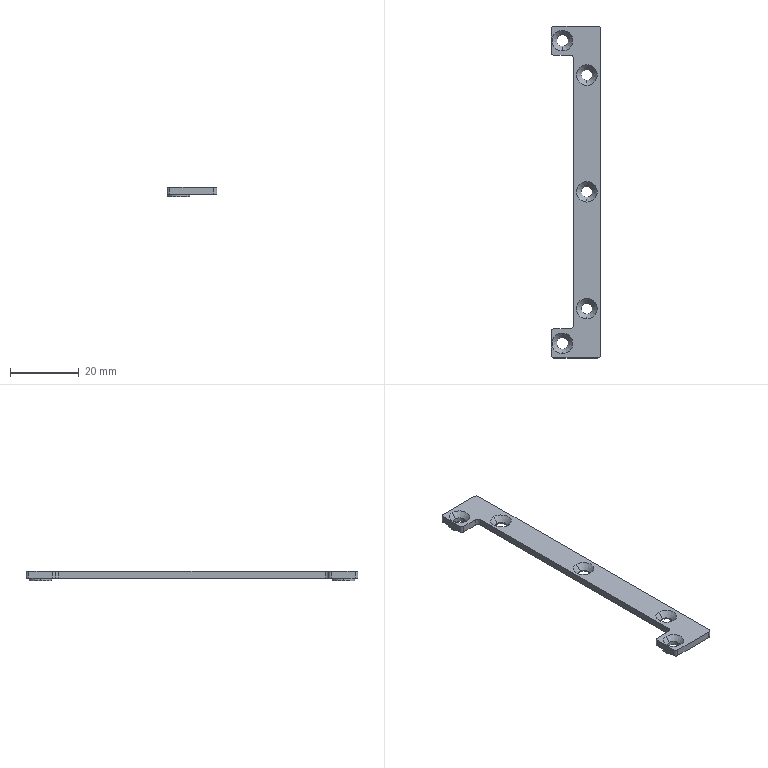Part | 1 solid | 44 faces | box 14.52 x 96.5 x 2.7 mm | volume 1629 mm3 | cylinder 22 | plane 12 | cone 10 | commonest cylinder face diameters 3.2 x6 1.6 x4 2 x4 3.4 x4 6.6 x4
STEP:
#1=CARTESIAN_POINT('',(-7.26,47.45,-2.));
#2=VERTEX_POINT('',#1);
#3=CARTESIAN_POINT('',(-7.26,44.,-2.));
#4=VERTEX_POINT('',#3);
#5=CARTESIAN_POINT('',(-7.26,47.45,-2.));
#6=DIRECTION('',(0.,-1.,0.));
#7=VECTOR('',#6,1000.);
#8=LINE('',#5,#7);
#9=EDGE_CURVE('',#2,#4,#8,.T.);
#10=ORIENTED_EDGE('',*,*,#9,.F.);
#11=CARTESIAN_POINT('',(-6.46,48.25,-2.));
#12=VERTEX_POINT('',#11);
#13=CARTESIAN_POINT('',(-6.46,47.45,-2.));
#14=DIRECTION('',(0.,0.,1.));
#15=DIRECTION('',(0.,1.,0.));
#16=AXIS2_PLACEMENT_3D('',#13,#14,#15);
#17=CIRCLE('',#16,0.8);
#18=EDGE_CURVE('',#12,#2,#17,.T.);
#19=ORIENTED_EDGE('',*,*,#18,.F.);
#20=CARTESIAN_POINT('',(6.26,48.25,-2.));
#21=VERTEX_POINT('',#20);
#22=CARTESIAN_POINT('',(6.26,48.25,-2.));
#23=DIRECTION('',(-1.,0.,0.));
#24=VECTOR('',#23,1000.);
#25=LINE('',#22,#24);
#26=EDGE_CURVE('',#21,#12,#25,.T.);
#27=ORIENTED_EDGE('',*,*,#26,.F.);
#28=CARTESIAN_POINT('',(7.26,47.25,-2.));
#29=VERTEX_POINT('',#28);
#30=CARTESIAN_POINT('',(6.26,47.25,-2.));
#31=DIRECTION('',(0.,0.,-1.));
#32=DIRECTION('',(0.,1.,0.));
#33=AXIS2_PLACEMENT_3D('',#30,#31,#32);
#34=CIRCLE('',#33,1.);
#35=EDGE_CURVE('',#21,#29,#34,.T.);
#36=ORIENTED_EDGE('',*,*,#35,.T.);
#37=CARTESIAN_POINT('',(7.26,-47.25,-2.));
#38=VERTEX_POINT('',#37);
#39=CARTESIAN_POINT('',(7.26,-47.25,-2.));
#40=DIRECTION('',(0.,1.,0.));
#41=VECTOR('',#40,1000.);
#42=LINE('',#39,#41);
#43=EDGE_CURVE('',#38,#29,#42,.T.);
#44=ORIENTED_EDGE('',*,*,#43,.F.);
#45=CARTESIAN_POINT('',(6.26,-48.25,-2.));
#46=VERTEX_POINT('',#45);
#47=CARTESIAN_POINT('',(6.26,-47.25,-2.));
#48=DIRECTION('',(0.,0.,-1.));
#49=DIRECTION('',(1.,0.,0.));
#50=AXIS2_PLACEMENT_3D('',#47,#48,#49);
#51=CIRCLE('',#50,1.);
#52=EDGE_CURVE('',#38,#46,#51,.T.);
#53=ORIENTED_EDGE('',*,*,#52,.T.);
#54=CARTESIAN_POINT('',(-6.46,-48.25,-2.));
#55=VERTEX_POINT('',#54);
#56=CARTESIAN_POINT('',(-6.46,-48.25,-2.));
#57=DIRECTION('',(1.,0.,0.));
#58=VECTOR('',#57,1000.);
#59=LINE('',#56,#58);
#60=EDGE_CURVE('',#55,#46,#59,.T.);
#61=ORIENTED_EDGE('',*,*,#60,.F.);
#62=CARTESIAN_POINT('',(-7.26,-47.45,-2.));
#63=VERTEX_POINT('',#62);
#64=CARTESIAN_POINT('',(-6.46,-47.45,-2.));
#65=DIRECTION('',(0.,0.,1.));
#66=DIRECTION('',(-1.,0.,0.));
#67=AXIS2_PLACEMENT_3D('',#64,#65,#66);
#68=CIRCLE('',#67,0.8);
#69=EDGE_CURVE('',#63,#55,#68,.T.);
#70=ORIENTED_EDGE('',*,*,#69,.F.);
#71=CARTESIAN_POINT('',(-7.26,-44.,-2.));
#72=VERTEX_POINT('',#71);
#73=CARTESIAN_POINT('',(-7.26,-44.,-2.));
#74=DIRECTION('',(0.,-1.,0.));
#75=VECTOR('',#74,1000.);
#76=LINE('',#73,#75);
#77=EDGE_CURVE('',#72,#63,#76,.T.);
#78=ORIENTED_EDGE('',*,*,#77,.F.);
#79=CARTESIAN_POINT('',(-0.66,-44.,-2.));
#80=VERTEX_POINT('',#79);
#81=CARTESIAN_POINT('',(-3.96,-44.,-2.));
#82=DIRECTION('',(0.,0.,-1.));
#83=DIRECTION('',(1.,0.,0.));
#84=AXIS2_PLACEMENT_3D('',#81,#82,#83);
#85=CIRCLE('',#84,3.3);
#86=EDGE_CURVE('',#80,#72,#85,.T.);
#87=ORIENTED_EDGE('',*,*,#86,.F.);
#88=CARTESIAN_POINT('',(-3.96,-44.,-2.));
#89=DIRECTION('',(0.,0.,-1.));
#90=DIRECTION('',(-1.,0.,0.));
#91=AXIS2_PLACEMENT_3D('',#88,#89,#90);
#92=CIRCLE('',#91,3.3);
#93=EDGE_CURVE('',#72,#80,#92,.T.);
#94=ORIENTED_EDGE('',*,*,#93,.F.);
#95=CARTESIAN_POINT('',(-7.26,-40.55,-2.));
#96=VERTEX_POINT('',#95);
#97=CARTESIAN_POINT('',(-7.26,-40.55,-2.));
#98=DIRECTION('',(0.,-1.,0.));
#99=VECTOR('',#98,1000.);
#100=LINE('',#97,#99);
#101=EDGE_CURVE('',#96,#72,#100,.T.);
#102=ORIENTED_EDGE('',*,*,#101,.F.);
#103=CARTESIAN_POINT('',(-6.46,-39.75,-2.));
#104=VERTEX_POINT('',#103);
#105=CARTESIAN_POINT('',(-6.46,-40.55,-2.));
#106=DIRECTION('',(0.,0.,1.));
#107=DIRECTION('',(0.,1.,0.));
#108=AXIS2_PLACEMENT_3D('',#105,#106,#107);
#109=CIRCLE('',#108,0.8);
#110=EDGE_CURVE('',#104,#96,#109,.T.);
#111=ORIENTED_EDGE('',*,*,#110,.F.);
#112=CARTESIAN_POINT('',(-1.66,-39.75,-2.));
#113=VERTEX_POINT('',#112);
#114=CARTESIAN_POINT('',(-1.66,-39.75,-2.));
#115=DIRECTION('',(-1.,0.,0.));
#116=VECTOR('',#115,1000.);
#117=LINE('',#114,#116);
#118=EDGE_CURVE('',#113,#104,#117,.T.);
#119=ORIENTED_EDGE('',*,*,#118,.F.);
#120=CARTESIAN_POINT('',(-0.66,-38.75,-2.));
#121=VERTEX_POINT('',#120);
#122=CARTESIAN_POINT('',(-1.66,-38.75,-2.));
#123=DIRECTION('',(0.,0.,1.));
#124=DIRECTION('',(0.,-1.,0.));
#125=AXIS2_PLACEMENT_3D('',#122,#123,#124);
#126=CIRCLE('',#125,1.);
#127=EDGE_CURVE('',#113,#121,#126,.T.);
#128=ORIENTED_EDGE('',*,*,#127,.T.);
#129=CARTESIAN_POINT('',(-0.66,38.75,-2.));
#130=VERTEX_POINT('',#129);
#131=CARTESIAN_POINT('',(-0.66,38.75,-2.));
#132=DIRECTION('',(0.,-1.,0.));
#133=VECTOR('',#132,1000.);
#134=LINE('',#131,#133);
#135=EDGE_CURVE('',#130,#121,#134,.T.);
#136=ORIENTED_EDGE('',*,*,#135,.F.);
#137=CARTESIAN_POINT('',(-1.66,39.75,-2.));
#138=VERTEX_POINT('',#137);
#139=CARTESIAN_POINT('',(-1.66,38.75,-2.));
#140=DIRECTION('',(0.,0.,1.));
#141=DIRECTION('',(1.,0.,0.));
#142=AXIS2_PLACEMENT_3D('',#139,#140,#141);
#143=CIRCLE('',#142,1.);
#144=EDGE_CURVE('',#130,#138,#143,.T.);
#145=ORIENTED_EDGE('',*,*,#144,.T.);
#146=CARTESIAN_POINT('',(-6.46,39.75,-2.));
#147=VERTEX_POINT('',#146);
#148=CARTESIAN_POINT('',(-6.46,39.75,-2.));
#149=DIRECTION('',(1.,0.,0.));
#150=VECTOR('',#149,1000.);
#151=LINE('',#148,#150);
#152=EDGE_CURVE('',#147,#138,#151,.T.);
#153=ORIENTED_EDGE('',*,*,#152,.F.);
#154=CARTESIAN_POINT('',(-7.26,40.55,-2.));
#155=VERTEX_POINT('',#154);
#156=CARTESIAN_POINT('',(-6.46,40.55,-2.));
#157=DIRECTION('',(0.,0.,1.));
#158=DIRECTION('',(-1.,0.,0.));
#159=AXIS2_PLACEMENT_3D('',#156,#157,#158);
#160=CIRCLE('',#159,0.8);
#161=EDGE_CURVE('',#155,#147,#160,.T.);
#162=ORIENTED_EDGE('',*,*,#161,.F.);
#163=CARTESIAN_POINT('',(-7.26,44.,-2.));
#164=DIRECTION('',(0.,-1.,0.));
#165=VECTOR('',#164,1000.);
#166=LINE('',#163,#165);
#167=EDGE_CURVE('',#4,#155,#166,.T.);
#168=ORIENTED_EDGE('',*,*,#167,.F.);
#169=CARTESIAN_POINT('',(-0.66,44.,-2.));
#170=VERTEX_POINT('',#169);
#171=CARTESIAN_POINT('',(-3.96,44.,-2.));
#172=DIRECTION('',(0.,0.,-1.));
#173=DIRECTION('',(1.,0.,0.));
#174=AXIS2_PLACEMENT_3D('',#171,#172,#173);
#175=CIRCLE('',#174,3.3);
#176=EDGE_CURVE('',#170,#4,#175,.T.);
#177=ORIENTED_EDGE('',*,*,#176,.F.);
#178=CARTESIAN_POINT('',(-3.96,44.,-2.));
#179=DIRECTION('',(0.,0.,-1.));
#180=DIRECTION('',(-1.,0.,0.));
#181=AXIS2_PLACEMENT_3D('',#178,#179,#180);
#182=CIRCLE('',#181,3.3);
#183=EDGE_CURVE('',#4,#170,#182,.T.);
#184=ORIENTED_EDGE('',*,*,#183,.F.);
#185=EDGE_LOOP('',(#10,#19,#27,#36,#44,#53,#61,#70,#78,#87,#94,#102,#111,#119,#128,#136,#145,#153,#162,#168,#177,#184));
#186=FACE_BOUND('',#185,.T.);
#187=CARTESIAN_POINT('',(1.55,0.05,-2.));
#188=VERTEX_POINT('',#187);
#189=CARTESIAN_POINT('',(4.75,0.05,-2.));
#190=VERTEX_POINT('',#189);
#191=CARTESIAN_POINT('',(3.15,0.05,-2.));
#192=DIRECTION('',(0.,0.,1.));
#193=DIRECTION('',(-1.,0.,0.));
#194=AXIS2_PLACEMENT_3D('',#191,#192,#193);
#195=CIRCLE('',#194,1.6);
#196=EDGE_CURVE('',#188,#190,#195,.T.);
#197=ORIENTED_EDGE('',*,*,#196,.T.);
#198=CARTESIAN_POINT('',(3.15,0.05,-2.));
#199=DIRECTION('',(0.,0.,1.));
#200=DIRECTION('',(1.,0.,0.));
#201=AXIS2_PLACEMENT_3D('',#198,#199,#200);
#202=CIRCLE('',#201,1.6);
#203=EDGE_CURVE('',#190,#188,#202,.T.);
#204=ORIENTED_EDGE('',*,*,#203,.T.);
#205=EDGE_LOOP('',(#197,#204));
#206=FACE_BOUND('',#205,.T.);
#207=CARTESIAN_POINT('',(1.55,-33.9,-2.));
#208=VERTEX_POINT('',#207);
#209=CARTESIAN_POINT('',(4.75,-33.9,-2.));
#210=VERTEX_POINT('',#209);
#211=CARTESIAN_POINT('',(3.15,-33.9,-2.));
#212=DIRECTION('',(0.,0.,1.));
#213=DIRECTION('',(-1.,0.,0.));
#214=AXIS2_PLACEMENT_3D('',#211,#212,#213);
#215=CIRCLE('',#214,1.6);
#216=EDGE_CURVE('',#208,#210,#215,.T.);
#217=ORIENTED_EDGE('',*,*,#216,.T.);
#218=CARTESIAN_POINT('',(3.15,-33.9,-2.));
#219=DIRECTION('',(0.,0.,1.));
#220=DIRECTION('',(1.,0.,0.));
#221=AXIS2_PLACEMENT_3D('',#218,#219,#220);
#222=CIRCLE('',#221,1.6);
#223=EDGE_CURVE('',#210,#208,#222,.T.);
#224=ORIENTED_EDGE('',*,*,#223,.T.);
#225=EDGE_LOOP('',(#217,#224));
#226=FACE_BOUND('',#225,.T.);
#227=CARTESIAN_POINT('',(1.55,34.,-2.));
#228=VERTEX_POINT('',#227);
#229=CARTESIAN_POINT('',(4.75,34.,-2.));
#230=VERTEX_POINT('',#229);
#231=CARTESIAN_POINT('',(3.15,34.,-2.));
#232=DIRECTION('',(0.,0.,1.));
#233=DIRECTION('',(-1.,0.,0.));
#234=AXIS2_PLACEMENT_3D('',#231,#232,#233);
#235=CIRCLE('',#234,1.6);
#236=EDGE_CURVE('',#228,#230,#235,.T.);
#237=ORIENTED_EDGE('',*,*,#236,.T.);
#238=CARTESIAN_POINT('',(3.15,34.,-2.));
#239=DIRECTION('',(0.,0.,1.));
#240=DIRECTION('',(1.,0.,0.));
#241=AXIS2_PLACEMENT_3D('',#238,#239,#240);
#242=CIRCLE('',#241,1.6);
#243=EDGE_CURVE('',#230,#228,#242,.T.);
#244=ORIENTED_EDGE('',*,*,#243,.T.);
#245=EDGE_LOOP('',(#237,#244));
#246=FACE_BOUND('',#245,.T.);
#247=CARTESIAN_POINT('',(-100.96,0.05,-2.));
#248=DIRECTION('',(0.,0.,1.));
#249=DIRECTION('',(-1.,0.,0.));
#250=AXIS2_PLACEMENT_3D('',#247,#248,#249);
#251=PLANE('',#250);
#252=ADVANCED_FACE('',(#186,#206,#226,#246),#251,.F.);
#253=CARTESIAN_POINT('',(1.55,34.,-1.68));
#254=VERTEX_POINT('',#253);
#255=CARTESIAN_POINT('',(1.55,34.,-2.));
#256=DIRECTION('',(0.,0.,1.));
#257=VECTOR('',#256,1000.);
#258=LINE('',#255,#257);
#259=EDGE_CURVE('',#254,#228,#258,.F.);
#260=ORIENTED_EDGE('',*,*,#259,.T.);
#261=ORIENTED_EDGE('',*,*,#243,.F.);
#262=CARTESIAN_POINT('',(4.75,34.,-1.68));
#263=VERTEX_POINT('',#262);
#264=CARTESIAN_POINT('',(4.75,34.,-2.));
#265=DIRECTION('',(0.,0.,1.));
#266=VECTOR('',#265,1000.);
#267=LINE('',#264,#266);
#268=EDGE_CURVE('',#263,#230,#267,.F.);
#269=ORIENTED_EDGE('',*,*,#268,.F.);
#270=CARTESIAN_POINT('',(3.15,35.6,-1.68));
#271=VERTEX_POINT('',#270);
#272=CARTESIAN_POINT('',(3.15,34.,-1.68));
#273=DIRECTION('',(0.,0.,1.));
#274=DIRECTION('',(1.,0.,0.));
#275=AXIS2_PLACEMENT_3D('',#272,#273,#274);
#276=CIRCLE('',#275,1.6);
#277=EDGE_CURVE('',#263,#271,#276,.T.);
#278=ORIENTED_EDGE('',*,*,#277,.T.);
#279=CARTESIAN_POINT('',(3.15,34.,-1.68));
#280=DIRECTION('',(0.,0.,1.));
#281=DIRECTION('',(0.,1.,0.));
#282=AXIS2_PLACEMENT_3D('',#279,#280,#281);
#283=CIRCLE('',#282,1.6);
#284=EDGE_CURVE('',#271,#254,#283,.T.);
#285=ORIENTED_EDGE('',*,*,#284,.T.);
#286=EDGE_LOOP('',(#260,#261,#269,#278,#285));
#287=FACE_BOUND('',#286,.T.);
#288=CARTESIAN_POINT('',(3.15,34.,-39.015));
#289=DIRECTION('',(0.,0.,1.));
#290=DIRECTION('',(-1.,0.,0.));
#291=AXIS2_PLACEMENT_3D('',#288,#289,#290);
#292=CYLINDRICAL_SURFACE('',#291,1.6);
#293=ADVANCED_FACE('',(#287),#292,.F.);
#294=CARTESIAN_POINT('',(3.15,32.4,-1.68));
#295=VERTEX_POINT('',#294);
#296=CARTESIAN_POINT('',(3.15,31.,0.));
#297=VERTEX_POINT('',#296);
#298=CARTESIAN_POINT('',(3.15,32.4,-1.68));
#299=DIRECTION('',(0.,-0.6402,0.7682));
#300=VECTOR('',#299,1000.);
#301=LINE('',#298,#300);
#302=EDGE_CURVE('',#295,#297,#301,.T.);
#303=ORIENTED_EDGE('',*,*,#302,.F.);
#304=CARTESIAN_POINT('',(3.15,34.,-1.68));
#305=DIRECTION('',(0.,0.,1.));
#306=DIRECTION('',(-1.,0.,0.));
#307=AXIS2_PLACEMENT_3D('',#304,#305,#306);
#308=CIRCLE('',#307,1.6);
#309=EDGE_CURVE('',#254,#295,#308,.T.);
#310=ORIENTED_EDGE('',*,*,#309,.F.);
#311=ORIENTED_EDGE('',*,*,#284,.F.);
#312=CARTESIAN_POINT('',(3.15,37.,0.));
#313=VERTEX_POINT('',#312);
#314=CARTESIAN_POINT('',(3.15,35.6,-1.68));
#315=DIRECTION('',(0.,0.6402,0.7682));
#316=VECTOR('',#315,1000.);
#317=LINE('',#314,#316);
#318=EDGE_CURVE('',#271,#313,#317,.T.);
#319=ORIENTED_EDGE('',*,*,#318,.T.);
#320=CARTESIAN_POINT('',(3.15,34.,0.));
#321=DIRECTION('',(0.,0.,-1.));
#322=DIRECTION('',(0.,-1.,0.));
#323=AXIS2_PLACEMENT_3D('',#320,#321,#322);
#324=CIRCLE('',#323,3.);
#325=EDGE_CURVE('',#297,#313,#324,.T.);
#326=ORIENTED_EDGE('',*,*,#325,.F.);
#327=EDGE_LOOP('',(#303,#310,#311,#319,#326));
#328=FACE_BOUND('',#327,.T.);
#329=CARTESIAN_POINT('',(3.15,34.,-0.84));
#330=DIRECTION('',(0.,0.,1.));
#331=DIRECTION('',(0.,1.,0.));
#332=AXIS2_PLACEMENT_3D('',#329,#330,#331);
#333=CONICAL_SURFACE('',#332,2.3,0.6947);
#334=ADVANCED_FACE('',(#328),#333,.F.);
#335=CARTESIAN_POINT('',(6.26,48.25,0.));
#336=VERTEX_POINT('',#335);
#337=CARTESIAN_POINT('',(-6.46,48.25,0.));
#338=VERTEX_POINT('',#337);
#339=CARTESIAN_POINT('',(6.26,48.25,0.));
#340=DIRECTION('',(-1.,0.,0.));
#341=VECTOR('',#340,1000.);
#342=LINE('',#339,#341);
#343=EDGE_CURVE('',#336,#338,#342,.T.);
#344=ORIENTED_EDGE('',*,*,#343,.T.);
#345=CARTESIAN_POINT('',(-7.26,47.45,0.));
#346=VERTEX_POINT('',#345);
#347=CARTESIAN_POINT('',(-6.46,47.45,0.));
#348=DIRECTION('',(0.,0.,1.));
#349=DIRECTION('',(0.,1.,0.));
#350=AXIS2_PLACEMENT_3D('',#347,#348,#349);
#351=CIRCLE('',#350,0.8);
#352=EDGE_CURVE('',#338,#346,#351,.T.);
#353=ORIENTED_EDGE('',*,*,#352,.T.);
#354=CARTESIAN_POINT('',(-7.26,40.55,0.));
#355=VERTEX_POINT('',#354);
#356=CARTESIAN_POINT('',(-7.26,47.45,0.));
#357=DIRECTION('',(0.,-1.,0.));
#358=VECTOR('',#357,1000.);
#359=LINE('',#356,#358);
#360=EDGE_CURVE('',#346,#355,#359,.T.);
#361=ORIENTED_EDGE('',*,*,#360,.T.);
#362=CARTESIAN_POINT('',(-6.46,39.75,0.));
#363=VERTEX_POINT('',#362);
#364=CARTESIAN_POINT('',(-6.46,40.55,0.));
#365=DIRECTION('',(0.,0.,1.));
#366=DIRECTION('',(-1.,0.,0.));
#367=AXIS2_PLACEMENT_3D('',#364,#365,#366);
#368=CIRCLE('',#367,0.8);
#369=EDGE_CURVE('',#355,#363,#368,.T.);
#370=ORIENTED_EDGE('',*,*,#369,.T.);
#371=CARTESIAN_POINT('',(-1.66,39.75,0.));
#372=VERTEX_POINT('',#371);
#373=CARTESIAN_POINT('',(-6.46,39.75,0.));
#374=DIRECTION('',(1.,0.,0.));
#375=VECTOR('',#374,1000.);
#376=LINE('',#373,#375);
#377=EDGE_CURVE('',#363,#372,#376,.T.);
#378=ORIENTED_EDGE('',*,*,#377,.T.);
#379=CARTESIAN_POINT('',(-0.66,38.75,0.));
#380=VERTEX_POINT('',#379);
#381=CARTESIAN_POINT('',(-1.66,38.75,0.));
#382=DIRECTION('',(0.,0.,-1.));
#383=DIRECTION('',(0.,1.,0.));
#384=AXIS2_PLACEMENT_3D('',#381,#382,#383);
#385=CIRCLE('',#384,1.);
#386=EDGE_CURVE('',#372,#380,#385,.T.);
#387=ORIENTED_EDGE('',*,*,#386,.T.);
#388=CARTESIAN_POINT('',(-0.66,-38.75,0.));
#389=VERTEX_POINT('',#388);
#390=CARTESIAN_POINT('',(-0.66,38.75,0.));
#391=DIRECTION('',(0.,-1.,0.));
#392=VECTOR('',#391,1000.);
#393=LINE('',#390,#392);
#394=EDGE_CURVE('',#380,#389,#393,.T.);
#395=ORIENTED_EDGE('',*,*,#394,.T.);
#396=CARTESIAN_POINT('',(-1.66,-39.75,0.));
#397=VERTEX_POINT('',#396);
#398=CARTESIAN_POINT('',(-1.66,-38.75,0.));
#399=DIRECTION('',(0.,0.,-1.));
#400=DIRECTION('',(1.,0.,0.));
#401=AXIS2_PLACEMENT_3D('',#398,#399,#400);
#402=CIRCLE('',#401,1.);
#403=EDGE_CURVE('',#389,#397,#402,.T.);
#404=ORIENTED_EDGE('',*,*,#403,.T.);
#405=CARTESIAN_POINT('',(-6.46,-39.75,0.));
#406=VERTEX_POINT('',#405);
#407=CARTESIAN_POINT('',(-1.66,-39.75,0.));
#408=DIRECTION('',(-1.,0.,0.));
#409=VECTOR('',#408,1000.);
#410=LINE('',#407,#409);
#411=EDGE_CURVE('',#397,#406,#410,.T.);
#412=ORIENTED_EDGE('',*,*,#411,.T.);
#413=CARTESIAN_POINT('',(-7.26,-40.55,0.));
#414=VERTEX_POINT('',#413);
#415=CARTESIAN_POINT('',(-6.46,-40.55,0.));
#416=DIRECTION('',(0.,0.,1.));
#417=DIRECTION('',(0.,1.,0.));
#418=AXIS2_PLACEMENT_3D('',#415,#416,#417);
#419=CIRCLE('',#418,0.8);
#420=EDGE_CURVE('',#406,#414,#419,.T.);
#421=ORIENTED_EDGE('',*,*,#420,.T.);
#422=CARTESIAN_POINT('',(-7.26,-47.45,0.));
#423=VERTEX_POINT('',#422);
#424=CARTESIAN_POINT('',(-7.26,-40.55,0.));
#425=DIRECTION('',(0.,-1.,0.));
#426=VECTOR('',#425,1000.);
#427=LINE('',#424,#426);
#428=EDGE_CURVE('',#414,#423,#427,.T.);
#429=ORIENTED_EDGE('',*,*,#428,.T.);
#430=CARTESIAN_POINT('',(-6.46,-48.25,0.));
#431=VERTEX_POINT('',#430);
#432=CARTESIAN_POINT('',(-6.46,-47.45,0.));
#433=DIRECTION('',(0.,0.,1.));
#434=DIRECTION('',(-1.,0.,0.));
#435=AXIS2_PLACEMENT_3D('',#432,#433,#434);
#436=CIRCLE('',#435,0.8);
#437=EDGE_CURVE('',#423,#431,#436,.T.);
#438=ORIENTED_EDGE('',*,*,#437,.T.);
#439=CARTESIAN_POINT('',(6.26,-48.25,0.));
#440=VERTEX_POINT('',#439);
#441=CARTESIAN_POINT('',(-6.46,-48.25,0.));
#442=DIRECTION('',(1.,0.,0.));
#443=VECTOR('',#442,1000.);
#444=LINE('',#441,#443);
#445=EDGE_CURVE('',#431,#440,#444,.T.);
#446=ORIENTED_EDGE('',*,*,#445,.T.);
#447=CARTESIAN_POINT('',(7.26,-47.25,0.));
#448=VERTEX_POINT('',#447);
#449=CARTESIAN_POINT('',(6.26,-47.25,0.));
#450=DIRECTION('',(0.,0.,1.));
#451=DIRECTION('',(0.,-1.,0.));
#452=AXIS2_PLACEMENT_3D('',#449,#450,#451);
#453=CIRCLE('',#452,1.);
#454=EDGE_CURVE('',#440,#448,#453,.T.);
#455=ORIENTED_EDGE('',*,*,#454,.T.);
#456=CARTESIAN_POINT('',(7.26,47.25,0.));
#457=VERTEX_POINT('',#456);
#458=CARTESIAN_POINT('',(7.26,-47.25,0.));
#459=DIRECTION('',(0.,1.,0.));
#460=VECTOR('',#459,1000.);
#461=LINE('',#458,#460);
#462=EDGE_CURVE('',#448,#457,#461,.T.);
#463=ORIENTED_EDGE('',*,*,#462,.T.);
#464=CARTESIAN_POINT('',(6.26,47.25,0.));
#465=DIRECTION('',(0.,0.,1.));
#466=DIRECTION('',(1.,0.,0.));
#467=AXIS2_PLACEMENT_3D('',#464,#465,#466);
#468=CIRCLE('',#467,1.);
#469=EDGE_CURVE('',#457,#336,#468,.T.);
#470=ORIENTED_EDGE('',*,*,#469,.T.);
#471=EDGE_LOOP('',(#344,#353,#361,#370,#378,#387,#395,#404,#412,#421,#429,#438,#446,#455,#463,#470));
#472=FACE_BOUND('',#471,.T.);
#473=CARTESIAN_POINT('',(-3.96,47.,0.));
#474=VERTEX_POINT('',#473);
#475=CARTESIAN_POINT('',(-3.96,41.,0.));
#476=VERTEX_POINT('',#475);
#477=CARTESIAN_POINT('',(-3.96,44.,0.));
#478=DIRECTION('',(0.,0.,-1.));
#479=DIRECTION('',(0.,1.,0.));
#480=AXIS2_PLACEMENT_3D('',#477,#478,#479);
#481=CIRCLE('',#480,3.);
#482=EDGE_CURVE('',#474,#476,#481,.T.);
#483=ORIENTED_EDGE('',*,*,#482,.T.);
#484=CARTESIAN_POINT('',(-3.96,44.,0.));
#485=DIRECTION('',(0.,0.,-1.));
#486=DIRECTION('',(0.,-1.,0.));
#487=AXIS2_PLACEMENT_3D('',#484,#485,#486);
#488=CIRCLE('',#487,3.);
#489=EDGE_CURVE('',#476,#474,#488,.T.);
#490=ORIENTED_EDGE('',*,*,#489,.T.);
#491=EDGE_LOOP('',(#483,#490));
#492=FACE_BOUND('',#491,.T.);
#493=CARTESIAN_POINT('',(3.15,34.,0.));
#494=DIRECTION('',(0.,0.,-1.));
#495=DIRECTION('',(0.,1.,0.));
#496=AXIS2_PLACEMENT_3D('',#493,#494,#495);
#497=CIRCLE('',#496,3.);
#498=EDGE_CURVE('',#313,#297,#497,.T.);
#499=ORIENTED_EDGE('',*,*,#498,.T.);
#500=ORIENTED_EDGE('',*,*,#325,.T.);
#501=EDGE_LOOP('',(#499,#500));
#502=FACE_BOUND('',#501,.T.);
#503=CARTESIAN_POINT('',(3.15,3.05,0.));
#504=VERTEX_POINT('',#503);
#505=CARTESIAN_POINT('',(3.15,-2.95,0.));
#506=VERTEX_POINT('',#505);
#507=CARTESIAN_POINT('',(3.15,0.05,0.));
#508=DIRECTION('',(0.,0.,-1.));
#509=DIRECTION('',(0.,1.,0.));
#510=AXIS2_PLACEMENT_3D('',#507,#508,#509);
#511=CIRCLE('',#510,3.);
#512=EDGE_CURVE('',#504,#506,#511,.T.);
#513=ORIENTED_EDGE('',*,*,#512,.T.);
#514=CARTESIAN_POINT('',(3.15,0.05,0.));
#515=DIRECTION('',(0.,0.,-1.));
#516=DIRECTION('',(0.,-1.,0.));
#517=AXIS2_PLACEMENT_3D('',#514,#515,#516);
#518=CIRCLE('',#517,3.);
#519=EDGE_CURVE('',#506,#504,#518,.T.);
#520=ORIENTED_EDGE('',*,*,#519,.T.);
#521=EDGE_LOOP('',(#513,#520));
#522=FACE_BOUND('',#521,.T.);
#523=CARTESIAN_POINT('',(-3.96,-41.,0.));
#524=VERTEX_POINT('',#523);
#525=CARTESIAN_POINT('',(-3.96,-47.,0.));
#526=VERTEX_POINT('',#525);
#527=CARTESIAN_POINT('',(-3.96,-44.,0.));
#528=DIRECTION('',(0.,0.,-1.));
#529=DIRECTION('',(0.,1.,0.));
#530=AXIS2_PLACEMENT_3D('',#527,#528,#529);
#531=CIRCLE('',#530,3.);
#532=EDGE_CURVE('',#524,#526,#531,.T.);
#533=ORIENTED_EDGE('',*,*,#532,.T.);
#534=CARTESIAN_POINT('',(-3.96,-44.,0.));
#535=DIRECTION('',(0.,0.,-1.));
#536=DIRECTION('',(0.,-1.,0.));
#537=AXIS2_PLACEMENT_3D('',#534,#535,#536);
#538=CIRCLE('',#537,3.);
#539=EDGE_CURVE('',#526,#524,#538,.T.);
#540=ORIENTED_EDGE('',*,*,#539,.T.);
#541=EDGE_LOOP('',(#533,#540));
#542=FACE_BOUND('',#541,.T.);
#543=CARTESIAN_POINT('',(3.15,-30.9,0.));
#544=VERTEX_POINT('',#543);
#545=CARTESIAN_POINT('',(3.15,-36.9,0.));
#546=VERTEX_POINT('',#545);
#547=CARTESIAN_POINT('',(3.15,-33.9,0.));
#548=DIRECTION('',(0.,0.,-1.));
#549=DIRECTION('',(0.,1.,0.));
#550=AXIS2_PLACEMENT_3D('',#547,#548,#549);
#551=CIRCLE('',#550,3.);
#552=EDGE_CURVE('',#544,#546,#551,.T.);
#553=ORIENTED_EDGE('',*,*,#552,.T.);
#554=CARTESIAN_POINT('',(3.15,-33.9,0.));
#555=DIRECTION('',(0.,0.,-1.));
#556=DIRECTION('',(0.,-1.,0.));
#557=AXIS2_PLACEMENT_3D('',#554,#555,#556);
#558=CIRCLE('',#557,3.);
#559=EDGE_CURVE('',#546,#544,#558,.T.);
#560=ORIENTED_EDGE('',*,*,#559,.T.);
#561=EDGE_LOOP('',(#553,#560));
#562=FACE_BOUND('',#561,.T.);
#563=CARTESIAN_POINT('',(-100.96,0.05,0.));
#564=DIRECTION('',(0.,0.,1.));
#565=DIRECTION('',(-1.,0.,0.));
#566=AXIS2_PLACEMENT_3D('',#563,#564,#565);
#567=PLANE('',#566);
#568=ADVANCED_FACE('',(#472,#492,#502,#522,#542,#562),#567,.T.);
#569=CARTESIAN_POINT('',(6.26,48.25,0.));
#570=DIRECTION('',(0.,0.,-1.));
#571=VECTOR('',#570,1000.);
#572=LINE('',#569,#571);
#573=EDGE_CURVE('',#336,#21,#572,.T.);
#574=ORIENTED_EDGE('',*,*,#573,.F.);
#575=ORIENTED_EDGE('',*,*,#469,.F.);
#576=CARTESIAN_POINT('',(7.26,47.25,0.));
#577=DIRECTION('',(0.,0.,-1.));
#578=VECTOR('',#577,1000.);
#579=LINE('',#576,#578);
#580=EDGE_CURVE('',#457,#29,#579,.T.);
#581=ORIENTED_EDGE('',*,*,#580,.T.);
#582=ORIENTED_EDGE('',*,*,#35,.F.);
#583=EDGE_LOOP('',(#574,#575,#581,#582));
#584=FACE_BOUND('',#583,.T.);
#585=CARTESIAN_POINT('',(6.26,47.25,19.222));
#586=DIRECTION('',(0.,0.,-1.));
#587=DIRECTION('',(0.,-1.,0.));
#588=AXIS2_PLACEMENT_3D('',#585,#586,#587);
#589=CYLINDRICAL_SURFACE('',#588,1.);
#590=ADVANCED_FACE('',(#584),#589,.T.);
#591=ORIENTED_EDGE('',*,*,#462,.F.);
#592=CARTESIAN_POINT('',(7.26,-47.25,0.));
#593=DIRECTION('',(0.,0.,-1.));
#594=VECTOR('',#593,1000.);
#595=LINE('',#592,#594);
#596=EDGE_CURVE('',#448,#38,#595,.T.);
#597=ORIENTED_EDGE('',*,*,#596,.T.);
#598=ORIENTED_EDGE('',*,*,#43,.T.);
#599=ORIENTED_EDGE('',*,*,#580,.F.);
#600=EDGE_LOOP('',(#591,#597,#598,#599));
#601=FACE_BOUND('',#600,.T.);
#602=CARTESIAN_POINT('',(7.26,-48.45,-2.));
#603=DIRECTION('',(1.,0.,0.));
#604=DIRECTION('',(0.,-1.,0.));
#605=AXIS2_PLACEMENT_3D('',#602,#603,#604);
#606=PLANE('',#605);
#607=ADVANCED_FACE('',(#601),#606,.T.);
#608=ORIENTED_EDGE('',*,*,#596,.F.);
#609=ORIENTED_EDGE('',*,*,#454,.F.);
#610=CARTESIAN_POINT('',(6.26,-48.25,0.));
#611=DIRECTION('',(0.,0.,-1.));
#612=VECTOR('',#611,1000.);
#613=LINE('',#610,#612);
#614=EDGE_CURVE('',#440,#46,#613,.T.);
#615=ORIENTED_EDGE('',*,*,#614,.T.);
#616=ORIENTED_EDGE('',*,*,#52,.F.);
#617=EDGE_LOOP('',(#608,#609,#615,#616));
#618=FACE_BOUND('',#617,.T.);
#619=CARTESIAN_POINT('',(6.26,-47.25,19.222));
#620=DIRECTION('',(0.,0.,-1.));
#621=DIRECTION('',(-1.,0.,0.));
#622=AXIS2_PLACEMENT_3D('',#619,#620,#621);
#623=CYLINDRICAL_SURFACE('',#622,1.);
#624=ADVANCED_FACE('',(#618),#623,.T.);
#625=ORIENTED_EDGE('',*,*,#445,.F.);
#626=CARTESIAN_POINT('',(-6.46,-48.25,-2.));
#627=DIRECTION('',(0.,0.,1.));
#628=VECTOR('',#627,1000.);
#629=LINE('',#626,#628);
#630=EDGE_CURVE('',#55,#431,#629,.T.);
#631=ORIENTED_EDGE('',*,*,#630,.F.);
#632=ORIENTED_EDGE('',*,*,#60,.T.);
#633=ORIENTED_EDGE('',*,*,#614,.F.);
#634=EDGE_LOOP('',(#625,#631,#632,#633));
#635=FACE_BOUND('',#634,.T.);
#636=CARTESIAN_POINT('',(-6.46,-48.25,-2.));
#637=DIRECTION('',(0.,-1.,0.));
#638=DIRECTION('',(-1.,0.,0.));
#639=AXIS2_PLACEMENT_3D('',#636,#637,#638);
#640=PLANE('',#639);
#641=ADVANCED_FACE('',(#635),#640,.T.);
#642=ORIENTED_EDGE('',*,*,#630,.T.);
#643=ORIENTED_EDGE('',*,*,#437,.F.);
#644=CARTESIAN_POINT('',(-7.26,-47.45,-2.));
#645=DIRECTION('',(0.,0.,1.));
#646=VECTOR('',#645,1000.);
#647=LINE('',#644,#646);
#648=EDGE_CURVE('',#63,#423,#647,.T.);
#649=ORIENTED_EDGE('',*,*,#648,.F.);
#650=ORIENTED_EDGE('',*,*,#69,.T.);
#651=EDGE_LOOP('',(#642,#643,#649,#650));
#652=FACE_BOUND('',#651,.T.);
#653=CARTESIAN_POINT('',(-6.46,-47.45,-2.));
#654=DIRECTION('',(0.,0.,1.));
#655=DIRECTION('',(-1.,0.,0.));
#656=AXIS2_PLACEMENT_3D('',#653,#654,#655);
#657=CYLINDRICAL_SURFACE('',#656,0.8);
#658=ADVANCED_FACE('',(#652),#657,.T.);
#659=ORIENTED_EDGE('',*,*,#77,.T.);
#660=ORIENTED_EDGE('',*,*,#648,.T.);
#661=ORIENTED_EDGE('',*,*,#428,.F.);
#662=CARTESIAN_POINT('',(-7.26,-40.55,-2.));
#663=DIRECTION('',(0.,0.,1.));
#664=VECTOR('',#663,1000.);
#665=LINE('',#662,#664);
#666=EDGE_CURVE('',#96,#414,#665,.T.);
#667=ORIENTED_EDGE('',*,*,#666,.F.);
#668=ORIENTED_EDGE('',*,*,#101,.T.);
#669=EDGE_LOOP('',(#659,#660,#661,#667,#668));
#670=FACE_BOUND('',#669,.T.);
#671=CARTESIAN_POINT('',(-7.26,-40.55,-2.));
#672=DIRECTION('',(-1.,0.,0.));
#673=DIRECTION('',(0.,1.,0.));
#674=AXIS2_PLACEMENT_3D('',#671,#672,#673);
#675=PLANE('',#674);
#676=ADVANCED_FACE('',(#670),#675,.T.);
#677=ORIENTED_EDGE('',*,*,#666,.T.);
#678=ORIENTED_EDGE('',*,*,#420,.F.);
#679=CARTESIAN_POINT('',(-6.46,-39.75,-2.));
#680=DIRECTION('',(0.,0.,1.));
#681=VECTOR('',#680,1000.);
#682=LINE('',#679,#681);
#683=EDGE_CURVE('',#104,#406,#682,.T.);
#684=ORIENTED_EDGE('',*,*,#683,.F.);
#685=ORIENTED_EDGE('',*,*,#110,.T.);
#686=EDGE_LOOP('',(#677,#678,#684,#685));
#687=FACE_BOUND('',#686,.T.);
#688=CARTESIAN_POINT('',(-6.46,-40.55,-2.));
#689=DIRECTION('',(0.,0.,1.));
#690=DIRECTION('',(-1.,0.,0.));
#691=AXIS2_PLACEMENT_3D('',#688,#689,#690);
#692=CYLINDRICAL_SURFACE('',#691,0.8);
#693=ADVANCED_FACE('',(#687),#692,.T.);
#694=ORIENTED_EDGE('',*,*,#118,.T.);
#695=ORIENTED_EDGE('',*,*,#683,.T.);
#696=ORIENTED_EDGE('',*,*,#411,.F.);
#697=CARTESIAN_POINT('',(-1.66,-39.75,-2.));
#698=DIRECTION('',(0.,0.,1.));
#699=VECTOR('',#698,1000.);
#700=LINE('',#697,#699);
#701=EDGE_CURVE('',#113,#397,#700,.T.);
#702=ORIENTED_EDGE('',*,*,#701,.F.);
#703=EDGE_LOOP('',(#694,#695,#696,#702));
#704=FACE_BOUND('',#703,.T.);
#705=CARTESIAN_POINT('',(-1.16,-39.75,-2.));
#706=DIRECTION('',(0.,1.,0.));
#707=DIRECTION('',(1.,0.,0.));
#708=AXIS2_PLACEMENT_3D('',#705,#706,#707);
#709=PLANE('',#708);
#710=ADVANCED_FACE('',(#704),#709,.T.);
#711=ORIENTED_EDGE('',*,*,#403,.F.);
#712=CARTESIAN_POINT('',(-0.66,-38.75,-2.));
#713=DIRECTION('',(0.,0.,1.));
#714=VECTOR('',#713,1000.);
#715=LINE('',#712,#714);
#716=EDGE_CURVE('',#121,#389,#715,.T.);
#717=ORIENTED_EDGE('',*,*,#716,.F.);
#718=ORIENTED_EDGE('',*,*,#127,.F.);
#719=ORIENTED_EDGE('',*,*,#701,.T.);
#720=EDGE_LOOP('',(#711,#717,#718,#719));
#721=FACE_BOUND('',#720,.T.);
#722=CARTESIAN_POINT('',(-1.66,-38.75,-22.622));
#723=DIRECTION('',(0.,0.,1.));
#724=DIRECTION('',(0.,1.,0.));
#725=AXIS2_PLACEMENT_3D('',#722,#723,#724);
#726=CYLINDRICAL_SURFACE('',#725,1.);
#727=ADVANCED_FACE('',(#721),#726,.F.);
#728=ORIENTED_EDGE('',*,*,#135,.T.);
#729=ORIENTED_EDGE('',*,*,#716,.T.);
#730=ORIENTED_EDGE('',*,*,#394,.F.);
#731=CARTESIAN_POINT('',(-0.66,38.75,-2.));
#732=DIRECTION('',(0.,0.,1.));
#733=VECTOR('',#732,1000.);
#734=LINE('',#731,#733);
#735=EDGE_CURVE('',#130,#380,#734,.T.);
#736=ORIENTED_EDGE('',*,*,#735,.F.);
#737=EDGE_LOOP('',(#728,#729,#730,#736));
#738=FACE_BOUND('',#737,.T.);
#739=CARTESIAN_POINT('',(-0.66,39.55,-2.));
#740=DIRECTION('',(-1.,0.,0.));
#741=DIRECTION('',(0.,1.,0.));
#742=AXIS2_PLACEMENT_3D('',#739,#740,#741);
#743=PLANE('',#742);
#744=ADVANCED_FACE('',(#738),#743,.T.);
#745=ORIENTED_EDGE('',*,*,#386,.F.);
#746=CARTESIAN_POINT('',(-1.66,39.75,-2.));
#747=DIRECTION('',(0.,0.,1.));
#748=VECTOR('',#747,1000.);
#749=LINE('',#746,#748);
#750=EDGE_CURVE('',#138,#372,#749,.T.);
#751=ORIENTED_EDGE('',*,*,#750,.F.);
#752=ORIENTED_EDGE('',*,*,#144,.F.);
#753=ORIENTED_EDGE('',*,*,#735,.T.);
#754=EDGE_LOOP('',(#745,#751,#752,#753));
#755=FACE_BOUND('',#754,.T.);
#756=CARTESIAN_POINT('',(-1.66,38.75,-22.622));
#757=DIRECTION('',(0.,0.,1.));
#758=DIRECTION('',(-1.,0.,0.));
#759=AXIS2_PLACEMENT_3D('',#756,#757,#758);
#760=CYLINDRICAL_SURFACE('',#759,1.);
#761=ADVANCED_FACE('',(#755),#760,.F.);
#762=ORIENTED_EDGE('',*,*,#377,.F.);
#763=CARTESIAN_POINT('',(-6.46,39.75,-2.));
#764=DIRECTION('',(0.,0.,1.));
#765=VECTOR('',#764,1000.);
#766=LINE('',#763,#765);
#767=EDGE_CURVE('',#147,#363,#766,.T.);
#768=ORIENTED_EDGE('',*,*,#767,.F.);
#769=ORIENTED_EDGE('',*,*,#152,.T.);
#770=ORIENTED_EDGE('',*,*,#750,.T.);
#771=EDGE_LOOP('',(#762,#768,#769,#770));
#772=FACE_BOUND('',#771,.T.);
#773=CARTESIAN_POINT('',(-6.46,39.75,-2.));
#774=DIRECTION('',(0.,-1.,0.));
#775=DIRECTION('',(-1.,0.,0.));
#776=AXIS2_PLACEMENT_3D('',#773,#774,#775);
#777=PLANE('',#776);
#778=ADVANCED_FACE('',(#772),#777,.T.);
#779=ORIENTED_EDGE('',*,*,#767,.T.);
#780=ORIENTED_EDGE('',*,*,#369,.F.);
#781=CARTESIAN_POINT('',(-7.26,40.55,-2.));
#782=DIRECTION('',(0.,0.,1.));
#783=VECTOR('',#782,1000.);
#784=LINE('',#781,#783);
#785=EDGE_CURVE('',#155,#355,#784,.T.);
#786=ORIENTED_EDGE('',*,*,#785,.F.);
#787=ORIENTED_EDGE('',*,*,#161,.T.);
#788=EDGE_LOOP('',(#779,#780,#786,#787));
#789=FACE_BOUND('',#788,.T.);
#790=CARTESIAN_POINT('',(-6.46,40.55,-2.));
#791=DIRECTION('',(0.,0.,1.));
#792=DIRECTION('',(-1.,0.,0.));
#793=AXIS2_PLACEMENT_3D('',#790,#791,#792);
#794=CYLINDRICAL_SURFACE('',#793,0.8);
#795=ADVANCED_FACE('',(#789),#794,.T.);
#796=ORIENTED_EDGE('',*,*,#167,.T.);
#797=ORIENTED_EDGE('',*,*,#785,.T.);
#798=ORIENTED_EDGE('',*,*,#360,.F.);
#799=CARTESIAN_POINT('',(-7.26,47.45,-2.));
#800=DIRECTION('',(0.,0.,1.));
#801=VECTOR('',#800,1000.);
#802=LINE('',#799,#801);
#803=EDGE_CURVE('',#2,#346,#802,.T.);
#804=ORIENTED_EDGE('',*,*,#803,.F.);
#805=ORIENTED_EDGE('',*,*,#9,.T.);
#806=EDGE_LOOP('',(#796,#797,#798,#804,#805));
#807=FACE_BOUND('',#806,.T.);
#808=CARTESIAN_POINT('',(-7.26,47.45,-2.));
#809=DIRECTION('',(-1.,0.,0.));
#810=DIRECTION('',(0.,1.,0.));
#811=AXIS2_PLACEMENT_3D('',#808,#809,#810);
#812=PLANE('',#811);
#813=ADVANCED_FACE('',(#807),#812,.T.);
#814=ORIENTED_EDGE('',*,*,#803,.T.);
#815=ORIENTED_EDGE('',*,*,#352,.F.);
#816=CARTESIAN_POINT('',(-6.46,48.25,-2.));
#817=DIRECTION('',(0.,0.,1.));
#818=VECTOR('',#817,1000.);
#819=LINE('',#816,#818);
#820=EDGE_CURVE('',#12,#338,#819,.T.);
#821=ORIENTED_EDGE('',*,*,#820,.F.);
#822=ORIENTED_EDGE('',*,*,#18,.T.);
#823=EDGE_LOOP('',(#814,#815,#821,#822));
#824=FACE_BOUND('',#823,.T.);
#825=CARTESIAN_POINT('',(-6.46,47.45,-2.));
#826=DIRECTION('',(0.,0.,1.));
#827=DIRECTION('',(-1.,0.,0.));
#828=AXIS2_PLACEMENT_3D('',#825,#826,#827);
#829=CYLINDRICAL_SURFACE('',#828,0.8);
#830=ADVANCED_FACE('',(#824),#829,.T.);
#831=ORIENTED_EDGE('',*,*,#26,.T.);
#832=ORIENTED_EDGE('',*,*,#820,.T.);
#833=ORIENTED_EDGE('',*,*,#343,.F.);
#834=ORIENTED_EDGE('',*,*,#573,.T.);
#835=EDGE_LOOP('',(#831,#832,#833,#834));
#836=FACE_BOUND('',#835,.T.);
#837=CARTESIAN_POINT('',(7.46,48.25,-2.));
#838=DIRECTION('',(0.,1.,0.));
#839=DIRECTION('',(1.,0.,0.));
#840=AXIS2_PLACEMENT_3D('',#837,#838,#839);
#841=PLANE('',#840);
#842=ADVANCED_FACE('',(#836),#841,.T.);
#843=CARTESIAN_POINT('',(-3.96,42.3,-1.56));
#844=VERTEX_POINT('',#843);
#845=CARTESIAN_POINT('',(-3.96,42.3,-1.56));
#846=DIRECTION('',(0.,-0.6402,0.7682));
#847=VECTOR('',#846,1000.);
#848=LINE('',#845,#847);
#849=EDGE_CURVE('',#844,#476,#848,.T.);
#850=ORIENTED_EDGE('',*,*,#849,.F.);
#851=CARTESIAN_POINT('',(-5.66,44.,-1.56));
#852=VERTEX_POINT('',#851);
#853=CARTESIAN_POINT('',(-3.96,44.,-1.56));
#854=DIRECTION('',(0.,0.,1.));
#855=DIRECTION('',(-1.,0.,0.));
#856=AXIS2_PLACEMENT_3D('',#853,#854,#855);
#857=CIRCLE('',#856,1.7);
#858=EDGE_CURVE('',#852,#844,#857,.T.);
#859=ORIENTED_EDGE('',*,*,#858,.F.);
#860=CARTESIAN_POINT('',(-3.96,45.7,-1.56));
#861=VERTEX_POINT('',#860);
#862=CARTESIAN_POINT('',(-3.96,44.,-1.56));
#863=DIRECTION('',(0.,0.,1.));
#864=DIRECTION('',(0.,1.,0.));
#865=AXIS2_PLACEMENT_3D('',#862,#863,#864);
#866=CIRCLE('',#865,1.7);
#867=EDGE_CURVE('',#861,#852,#866,.T.);
#868=ORIENTED_EDGE('',*,*,#867,.F.);
#869=CARTESIAN_POINT('',(-3.96,45.7,-1.56));
#870=DIRECTION('',(0.,0.6402,0.7682));
#871=VECTOR('',#870,1000.);
#872=LINE('',#869,#871);
#873=EDGE_CURVE('',#861,#474,#872,.T.);
#874=ORIENTED_EDGE('',*,*,#873,.T.);
#875=ORIENTED_EDGE('',*,*,#489,.F.);
#876=EDGE_LOOP('',(#850,#859,#868,#874,#875));
#877=FACE_BOUND('',#876,.T.);
#878=CARTESIAN_POINT('',(-3.96,44.,-0.78));
#879=DIRECTION('',(0.,0.,1.));
#880=DIRECTION('',(0.,1.,0.));
#881=AXIS2_PLACEMENT_3D('',#878,#879,#880);
#882=CONICAL_SURFACE('',#881,2.35,0.6947);
#883=ADVANCED_FACE('',(#877),#882,.F.);
#884=ORIENTED_EDGE('',*,*,#873,.F.);
#885=CARTESIAN_POINT('',(-2.26,44.,-1.56));
#886=VERTEX_POINT('',#885);
#887=CARTESIAN_POINT('',(-3.96,44.,-1.56));
#888=DIRECTION('',(0.,0.,1.));
#889=DIRECTION('',(1.,0.,0.));
#890=AXIS2_PLACEMENT_3D('',#887,#888,#889);
#891=CIRCLE('',#890,1.7);
#892=EDGE_CURVE('',#886,#861,#891,.T.);
#893=ORIENTED_EDGE('',*,*,#892,.F.);
#894=CARTESIAN_POINT('',(-3.96,44.,-1.56));
#895=DIRECTION('',(0.,0.,1.));
#896=DIRECTION('',(0.,-1.,0.));
#897=AXIS2_PLACEMENT_3D('',#894,#895,#896);
#898=CIRCLE('',#897,1.7);
#899=EDGE_CURVE('',#844,#886,#898,.T.);
#900=ORIENTED_EDGE('',*,*,#899,.F.);
#901=ORIENTED_EDGE('',*,*,#849,.T.);
#902=ORIENTED_EDGE('',*,*,#482,.F.);
#903=EDGE_LOOP('',(#884,#893,#900,#901,#902));
#904=FACE_BOUND('',#903,.T.);
#905=CARTESIAN_POINT('',(-3.96,44.,-0.78));
#906=DIRECTION('',(0.,0.,1.));
#907=DIRECTION('',(0.,1.,0.));
#908=AXIS2_PLACEMENT_3D('',#905,#906,#907);
#909=CONICAL_SURFACE('',#908,2.35,0.6947);
#910=ADVANCED_FACE('',(#904),#909,.F.);
#911=ORIENTED_EDGE('',*,*,#858,.T.);
#912=ORIENTED_EDGE('',*,*,#899,.T.);
#913=CARTESIAN_POINT('',(-2.26,44.,-2.7));
#914=VERTEX_POINT('',#913);
#915=CARTESIAN_POINT('',(-2.26,44.,-1.56));
#916=DIRECTION('',(0.,0.,-1.));
#917=VECTOR('',#916,1000.);
#918=LINE('',#915,#917);
#919=EDGE_CURVE('',#886,#914,#918,.T.);
#920=ORIENTED_EDGE('',*,*,#919,.T.);
#921=CARTESIAN_POINT('',(-5.66,44.,-2.7));
#922=VERTEX_POINT('',#921);
#923=CARTESIAN_POINT('',(-3.96,44.,-2.7));
#924=DIRECTION('',(0.,0.,1.));
#925=DIRECTION('',(-1.,0.,0.));
#926=AXIS2_PLACEMENT_3D('',#923,#924,#925);
#927=CIRCLE('',#926,1.7);
#928=EDGE_CURVE('',#922,#914,#927,.T.);
#929=ORIENTED_EDGE('',*,*,#928,.F.);
#930=CARTESIAN_POINT('',(-5.66,44.,-2.7));
#931=DIRECTION('',(0.,0.,1.));
#932=VECTOR('',#931,1000.);
#933=LINE('',#930,#932);
#934=EDGE_CURVE('',#922,#852,#933,.T.);
#935=ORIENTED_EDGE('',*,*,#934,.T.);
#936=EDGE_LOOP('',(#911,#912,#920,#929,#935));
#937=FACE_BOUND('',#936,.T.);
#938=CARTESIAN_POINT('',(-3.96,44.,-2.));
#939=DIRECTION('',(0.,0.,1.));
#940=DIRECTION('',(-1.,0.,0.));
#941=AXIS2_PLACEMENT_3D('',#938,#939,#940);
#942=CYLINDRICAL_SURFACE('',#941,1.7);
#943=ADVANCED_FACE('',(#937),#942,.F.);
#944=ORIENTED_EDGE('',*,*,#892,.T.);
#945=ORIENTED_EDGE('',*,*,#867,.T.);
#946=ORIENTED_EDGE('',*,*,#934,.F.);
#947=CARTESIAN_POINT('',(-3.96,44.,-2.7));
#948=DIRECTION('',(0.,0.,1.));
#949=DIRECTION('',(1.,0.,0.));
#950=AXIS2_PLACEMENT_3D('',#947,#948,#949);
#951=CIRCLE('',#950,1.7);
#952=EDGE_CURVE('',#914,#922,#951,.T.);
#953=ORIENTED_EDGE('',*,*,#952,.F.);
#954=ORIENTED_EDGE('',*,*,#919,.F.);
#955=EDGE_LOOP('',(#944,#945,#946,#953,#954));
#956=FACE_BOUND('',#955,.T.);
#957=CARTESIAN_POINT('',(-3.96,44.,-2.));
#958=DIRECTION('',(0.,0.,1.));
#959=DIRECTION('',(-1.,0.,0.));
#960=AXIS2_PLACEMENT_3D('',#957,#958,#959);
#961=CYLINDRICAL_SURFACE('',#960,1.7);
#962=ADVANCED_FACE('',(#956),#961,.F.);
#963=CARTESIAN_POINT('',(-0.66,44.,-2.7));
#964=VERTEX_POINT('',#963);
#965=CARTESIAN_POINT('',(-7.26,44.,-2.7));
#966=VERTEX_POINT('',#965);
#967=CARTESIAN_POINT('',(-3.96,44.,-2.7));
#968=DIRECTION('',(0.,0.,-1.));
#969=DIRECTION('',(1.,0.,0.));
#970=AXIS2_PLACEMENT_3D('',#967,#968,#969);
#971=CIRCLE('',#970,3.3);
#972=EDGE_CURVE('',#964,#966,#971,.T.);
#973=ORIENTED_EDGE('',*,*,#972,.T.);
#974=CARTESIAN_POINT('',(-3.96,44.,-2.7));
#975=DIRECTION('',(0.,0.,-1.));
#976=DIRECTION('',(-1.,0.,0.));
#977=AXIS2_PLACEMENT_3D('',#974,#975,#976);
#978=CIRCLE('',#977,3.3);
#979=EDGE_CURVE('',#966,#964,#978,.T.);
#980=ORIENTED_EDGE('',*,*,#979,.T.);
#981=EDGE_LOOP('',(#973,#980));
#982=FACE_BOUND('',#981,.T.);
#983=ORIENTED_EDGE('',*,*,#952,.T.);
#984=ORIENTED_EDGE('',*,*,#928,.T.);
#985=EDGE_LOOP('',(#983,#984));
#986=FACE_BOUND('',#985,.T.);
#987=CARTESIAN_POINT('',(-100.96,0.05,-2.7));
#988=DIRECTION('',(0.,0.,-1.));
#989=DIRECTION('',(1.,0.,0.));
#990=AXIS2_PLACEMENT_3D('',#987,#988,#989);
#991=PLANE('',#990);
#992=ADVANCED_FACE('',(#982,#986),#991,.T.);
#993=CARTESIAN_POINT('',(-0.66,-44.,-2.7));
#994=VERTEX_POINT('',#993);
#995=CARTESIAN_POINT('',(-7.26,-44.,-2.7));
#996=VERTEX_POINT('',#995);
#997=CARTESIAN_POINT('',(-3.96,-44.,-2.7));
#998=DIRECTION('',(0.,0.,-1.));
#999=DIRECTION('',(1.,0.,0.));
#1000=AXIS2_PLACEMENT_3D('',#997,#998,#999);
#1001=CIRCLE('',#1000,3.3);
#1002=EDGE_CURVE('',#994,#996,#1001,.T.);
#1003=ORIENTED_EDGE('',*,*,#1002,.T.);
#1004=CARTESIAN_POINT('',(-3.96,-44.,-2.7));
#1005=DIRECTION('',(0.,0.,-1.));
#1006=DIRECTION('',(-1.,0.,0.));
#1007=AXIS2_PLACEMENT_3D('',#1004,#1005,#1006);
#1008=CIRCLE('',#1007,3.3);
#1009=EDGE_CURVE('',#996,#994,#1008,.T.);
#1010=ORIENTED_EDGE('',*,*,#1009,.T.);
#1011=EDGE_LOOP('',(#1003,#1010));
#1012=FACE_BOUND('',#1011,.T.);
#1013=CARTESIAN_POINT('',(-2.26,-44.,-2.7));
#1014=VERTEX_POINT('',#1013);
#1015=CARTESIAN_POINT('',(-5.66,-44.,-2.7));
#1016=VERTEX_POINT('',#1015);
#1017=CARTESIAN_POINT('',(-3.96,-44.,-2.7));
#1018=DIRECTION('',(0.,0.,1.));
#1019=DIRECTION('',(1.,0.,0.));
#1020=AXIS2_PLACEMENT_3D('',#1017,#1018,#1019);
#1021=CIRCLE('',#1020,1.7);
#1022=EDGE_CURVE('',#1014,#1016,#1021,.T.);
#1023=ORIENTED_EDGE('',*,*,#1022,.T.);
#1024=CARTESIAN_POINT('',(-3.96,-44.,-2.7));
#1025=DIRECTION('',(0.,0.,1.));
#1026=DIRECTION('',(-1.,0.,0.));
#1027=AXIS2_PLACEMENT_3D('',#1024,#1025,#1026);
#1028=CIRCLE('',#1027,1.7);
#1029=EDGE_CURVE('',#1016,#1014,#1028,.T.);
#1030=ORIENTED_EDGE('',*,*,#1029,.T.);
#1031=EDGE_LOOP('',(#1023,#1030));
#1032=FACE_BOUND('',#1031,.T.);
#1033=CARTESIAN_POINT('',(-100.96,0.05,-2.7));
#1034=DIRECTION('',(0.,0.,-1.));
#1035=DIRECTION('',(1.,0.,0.));
#1036=AXIS2_PLACEMENT_3D('',#1033,#1034,#1035);
#1037=PLANE('',#1036);
#1038=ADVANCED_FACE('',(#1012,#1032),#1037,.T.);
#1039=CARTESIAN_POINT('',(-0.66,44.,-2.));
#1040=DIRECTION('',(0.,0.,-1.));
#1041=VECTOR('',#1040,1000.);
#1042=LINE('',#1039,#1041);
#1043=EDGE_CURVE('',#964,#170,#1042,.F.);
#1044=ORIENTED_EDGE('',*,*,#1043,.F.);
#1045=ORIENTED_EDGE('',*,*,#979,.F.);
#1046=CARTESIAN_POINT('',(-7.26,44.,-2.));
#1047=DIRECTION('',(0.,0.,-1.));
#1048=VECTOR('',#1047,1000.);
#1049=LINE('',#1046,#1048);
#1050=EDGE_CURVE('',#966,#4,#1049,.F.);
#1051=ORIENTED_EDGE('',*,*,#1050,.T.);
#1052=ORIENTED_EDGE('',*,*,#183,.T.);
#1053=EDGE_LOOP('',(#1044,#1045,#1051,#1052));
#1054=FACE_BOUND('',#1053,.T.);
#1055=CARTESIAN_POINT('',(-3.96,44.,-2.));
#1056=DIRECTION('',(0.,0.,-1.));
#1057=DIRECTION('',(1.,0.,0.));
#1058=AXIS2_PLACEMENT_3D('',#1055,#1056,#1057);
#1059=CYLINDRICAL_SURFACE('',#1058,3.3);
#1060=ADVANCED_FACE('',(#1054),#1059,.T.);
#1061=ORIENTED_EDGE('',*,*,#1050,.F.);
#1062=ORIENTED_EDGE('',*,*,#972,.F.);
#1063=ORIENTED_EDGE('',*,*,#1043,.T.);
#1064=ORIENTED_EDGE('',*,*,#176,.T.);
#1065=EDGE_LOOP('',(#1061,#1062,#1063,#1064));
#1066=FACE_BOUND('',#1065,.T.);
#1067=CARTESIAN_POINT('',(-3.96,44.,-2.));
#1068=DIRECTION('',(0.,0.,-1.));
#1069=DIRECTION('',(1.,0.,0.));
#1070=AXIS2_PLACEMENT_3D('',#1067,#1068,#1069);
#1071=CYLINDRICAL_SURFACE('',#1070,3.3);
#1072=ADVANCED_FACE('',(#1066),#1071,.T.);
#1073=CARTESIAN_POINT('',(-0.66,-44.,-2.));
#1074=DIRECTION('',(0.,0.,-1.));
#1075=VECTOR('',#1074,1000.);
#1076=LINE('',#1073,#1075);
#1077=EDGE_CURVE('',#994,#80,#1076,.F.);
#1078=ORIENTED_EDGE('',*,*,#1077,.F.);
#1079=ORIENTED_EDGE('',*,*,#1009,.F.);
#1080=CARTESIAN_POINT('',(-7.26,-44.,-2.));
#1081=DIRECTION('',(0.,0.,-1.));
#1082=VECTOR('',#1081,1000.);
#1083=LINE('',#1080,#1082);
#1084=EDGE_CURVE('',#996,#72,#1083,.F.);
#1085=ORIENTED_EDGE('',*,*,#1084,.T.);
#1086=ORIENTED_EDGE('',*,*,#93,.T.);
#1087=EDGE_LOOP('',(#1078,#1079,#1085,#1086));
#1088=FACE_BOUND('',#1087,.T.);
#1089=CARTESIAN_POINT('',(-3.96,-44.,-2.));
#1090=DIRECTION('',(0.,0.,-1.));
#1091=DIRECTION('',(1.,0.,0.));
#1092=AXIS2_PLACEMENT_3D('',#1089,#1090,#1091);
#1093=CYLINDRICAL_SURFACE('',#1092,3.3);
#1094=ADVANCED_FACE('',(#1088),#1093,.T.);
#1095=ORIENTED_EDGE('',*,*,#1084,.F.);
#1096=ORIENTED_EDGE('',*,*,#1002,.F.);
#1097=ORIENTED_EDGE('',*,*,#1077,.T.);
#1098=ORIENTED_EDGE('',*,*,#86,.T.);
#1099=EDGE_LOOP('',(#1095,#1096,#1097,#1098));
#1100=FACE_BOUND('',#1099,.T.);
#1101=CARTESIAN_POINT('',(-3.96,-44.,-2.));
#1102=DIRECTION('',(0.,0.,-1.));
#1103=DIRECTION('',(1.,0.,0.));
#1104=AXIS2_PLACEMENT_3D('',#1101,#1102,#1103);
#1105=CYLINDRICAL_SURFACE('',#1104,3.3);
#1106=ADVANCED_FACE('',(#1100),#1105,.T.);
#1107=CARTESIAN_POINT('',(-5.66,-44.,-1.56));
#1108=VERTEX_POINT('',#1107);
#1109=CARTESIAN_POINT('',(-3.96,-45.7,-1.56));
#1110=VERTEX_POINT('',#1109);
#1111=CARTESIAN_POINT('',(-3.96,-44.,-1.56));
#1112=DIRECTION('',(0.,0.,1.));
#1113=DIRECTION('',(-1.,0.,0.));
#1114=AXIS2_PLACEMENT_3D('',#1111,#1112,#1113);
#1115=CIRCLE('',#1114,1.7);
#1116=EDGE_CURVE('',#1108,#1110,#1115,.T.);
#1117=ORIENTED_EDGE('',*,*,#1116,.T.);
#1118=CARTESIAN_POINT('',(-2.26,-44.,-1.56));
#1119=VERTEX_POINT('',#1118);
#1120=CARTESIAN_POINT('',(-3.96,-44.,-1.56));
#1121=DIRECTION('',(0.,0.,1.));
#1122=DIRECTION('',(0.,-1.,0.));
#1123=AXIS2_PLACEMENT_3D('',#1120,#1121,#1122);
#1124=CIRCLE('',#1123,1.7);
#1125=EDGE_CURVE('',#1110,#1119,#1124,.T.);
#1126=ORIENTED_EDGE('',*,*,#1125,.T.);
#1127=CARTESIAN_POINT('',(-2.26,-44.,-1.56));
#1128=DIRECTION('',(0.,0.,-1.));
#1129=VECTOR('',#1128,1000.);
#1130=LINE('',#1127,#1129);
#1131=EDGE_CURVE('',#1119,#1014,#1130,.T.);
#1132=ORIENTED_EDGE('',*,*,#1131,.T.);
#1133=ORIENTED_EDGE('',*,*,#1029,.F.);
#1134=CARTESIAN_POINT('',(-5.66,-44.,-2.7));
#1135=DIRECTION('',(0.,0.,1.));
#1136=VECTOR('',#1135,1000.);
#1137=LINE('',#1134,#1136);
#1138=EDGE_CURVE('',#1016,#1108,#1137,.T.);
#1139=ORIENTED_EDGE('',*,*,#1138,.T.);
#1140=EDGE_LOOP('',(#1117,#1126,#1132,#1133,#1139));
#1141=FACE_BOUND('',#1140,.T.);
#1142=CARTESIAN_POINT('',(-3.96,-44.,-2.));
#1143=DIRECTION('',(0.,0.,1.));
#1144=DIRECTION('',(-1.,0.,0.));
#1145=AXIS2_PLACEMENT_3D('',#1142,#1143,#1144);
#1146=CYLINDRICAL_SURFACE('',#1145,1.7);
#1147=ADVANCED_FACE('',(#1141),#1146,.F.);
#1148=CARTESIAN_POINT('',(-3.96,-42.3,-1.56));
#1149=VERTEX_POINT('',#1148);
#1150=CARTESIAN_POINT('',(-3.96,-44.,-1.56));
#1151=DIRECTION('',(0.,0.,1.));
#1152=DIRECTION('',(1.,0.,0.));
#1153=AXIS2_PLACEMENT_3D('',#1150,#1151,#1152);
#1154=CIRCLE('',#1153,1.7);
#1155=EDGE_CURVE('',#1119,#1149,#1154,.T.);
#1156=ORIENTED_EDGE('',*,*,#1155,.T.);
#1157=CARTESIAN_POINT('',(-3.96,-44.,-1.56));
#1158=DIRECTION('',(0.,0.,1.));
#1159=DIRECTION('',(0.,1.,0.));
#1160=AXIS2_PLACEMENT_3D('',#1157,#1158,#1159);
#1161=CIRCLE('',#1160,1.7);
#1162=EDGE_CURVE('',#1149,#1108,#1161,.T.);
#1163=ORIENTED_EDGE('',*,*,#1162,.T.);
#1164=ORIENTED_EDGE('',*,*,#1138,.F.);
#1165=ORIENTED_EDGE('',*,*,#1022,.F.);
#1166=ORIENTED_EDGE('',*,*,#1131,.F.);
#1167=EDGE_LOOP('',(#1156,#1163,#1164,#1165,#1166));
#1168=FACE_BOUND('',#1167,.T.);
#1169=CARTESIAN_POINT('',(-3.96,-44.,-2.));
#1170=DIRECTION('',(0.,0.,1.));
#1171=DIRECTION('',(-1.,0.,0.));
#1172=AXIS2_PLACEMENT_3D('',#1169,#1170,#1171);
#1173=CYLINDRICAL_SURFACE('',#1172,1.7);
#1174=ADVANCED_FACE('',(#1168),#1173,.F.);
#1175=CARTESIAN_POINT('',(-3.96,-45.7,-1.56));
#1176=DIRECTION('',(0.,-0.6402,0.7682));
#1177=VECTOR('',#1176,1000.);
#1178=LINE('',#1175,#1177);
#1179=EDGE_CURVE('',#1110,#526,#1178,.T.);
#1180=ORIENTED_EDGE('',*,*,#1179,.F.);
#1181=ORIENTED_EDGE('',*,*,#1116,.F.);
#1182=ORIENTED_EDGE('',*,*,#1162,.F.);
#1183=CARTESIAN_POINT('',(-3.96,-42.3,-1.56));
#1184=DIRECTION('',(0.,0.6402,0.7682));
#1185=VECTOR('',#1184,1000.);
#1186=LINE('',#1183,#1185);
#1187=EDGE_CURVE('',#1149,#524,#1186,.T.);
#1188=ORIENTED_EDGE('',*,*,#1187,.T.);
#1189=ORIENTED_EDGE('',*,*,#539,.F.);
#1190=EDGE_LOOP('',(#1180,#1181,#1182,#1188,#1189));
#1191=FACE_BOUND('',#1190,.T.);
#1192=CARTESIAN_POINT('',(-3.96,-44.,-0.78));
#1193=DIRECTION('',(0.,0.,1.));
#1194=DIRECTION('',(0.,1.,0.));
#1195=AXIS2_PLACEMENT_3D('',#1192,#1193,#1194);
#1196=CONICAL_SURFACE('',#1195,2.35,0.6947);
#1197=ADVANCED_FACE('',(#1191),#1196,.F.);
#1198=ORIENTED_EDGE('',*,*,#1187,.F.);
#1199=ORIENTED_EDGE('',*,*,#1155,.F.);
#1200=ORIENTED_EDGE('',*,*,#1125,.F.);
#1201=ORIENTED_EDGE('',*,*,#1179,.T.);
#1202=ORIENTED_EDGE('',*,*,#532,.F.);
#1203=EDGE_LOOP('',(#1198,#1199,#1200,#1201,#1202));
#1204=FACE_BOUND('',#1203,.T.);
#1205=CARTESIAN_POINT('',(-3.96,-44.,-0.78));
#1206=DIRECTION('',(0.,0.,1.));
#1207=DIRECTION('',(0.,1.,0.));
#1208=AXIS2_PLACEMENT_3D('',#1205,#1206,#1207);
#1209=CONICAL_SURFACE('',#1208,2.35,0.6947);
#1210=ADVANCED_FACE('',(#1204),#1209,.F.);
#1211=ORIENTED_EDGE('',*,*,#318,.F.);
#1212=ORIENTED_EDGE('',*,*,#277,.F.);
#1213=CARTESIAN_POINT('',(3.15,34.,-1.68));
#1214=DIRECTION('',(0.,0.,1.));
#1215=DIRECTION('',(0.,-1.,0.));
#1216=AXIS2_PLACEMENT_3D('',#1213,#1214,#1215);
#1217=CIRCLE('',#1216,1.6);
#1218=EDGE_CURVE('',#295,#263,#1217,.T.);
#1219=ORIENTED_EDGE('',*,*,#1218,.F.);
#1220=ORIENTED_EDGE('',*,*,#302,.T.);
#1221=ORIENTED_EDGE('',*,*,#498,.F.);
#1222=EDGE_LOOP('',(#1211,#1212,#1219,#1220,#1221));
#1223=FACE_BOUND('',#1222,.T.);
#1224=CARTESIAN_POINT('',(3.15,34.,-0.84));
#1225=DIRECTION('',(0.,0.,1.));
#1226=DIRECTION('',(0.,1.,0.));
#1227=AXIS2_PLACEMENT_3D('',#1224,#1225,#1226);
#1228=CONICAL_SURFACE('',#1227,2.3,0.6947);
#1229=ADVANCED_FACE('',(#1223),#1228,.F.);
#1230=ORIENTED_EDGE('',*,*,#1218,.T.);
#1231=ORIENTED_EDGE('',*,*,#268,.T.);
#1232=ORIENTED_EDGE('',*,*,#236,.F.);
#1233=ORIENTED_EDGE('',*,*,#259,.F.);
#1234=ORIENTED_EDGE('',*,*,#309,.T.);
#1235=EDGE_LOOP('',(#1230,#1231,#1232,#1233,#1234));
#1236=FACE_BOUND('',#1235,.T.);
#1237=CARTESIAN_POINT('',(3.15,34.,-39.015));
#1238=DIRECTION('',(0.,0.,1.));
#1239=DIRECTION('',(-1.,0.,0.));
#1240=AXIS2_PLACEMENT_3D('',#1237,#1238,#1239);
#1241=CYLINDRICAL_SURFACE('',#1240,1.6);
#1242=ADVANCED_FACE('',(#1236),#1241,.F.);
#1243=CARTESIAN_POINT('',(3.15,-1.55,-1.68));
#1244=VERTEX_POINT('',#1243);
#1245=CARTESIAN_POINT('',(3.15,-1.55,-1.68));
#1246=DIRECTION('',(0.,-0.6402,0.7682));
#1247=VECTOR('',#1246,1000.);
#1248=LINE('',#1245,#1247);
#1249=EDGE_CURVE('',#1244,#506,#1248,.T.);
#1250=ORIENTED_EDGE('',*,*,#1249,.F.);
#1251=CARTESIAN_POINT('',(1.55,0.05,-1.68));
#1252=VERTEX_POINT('',#1251);
#1253=CARTESIAN_POINT('',(3.15,0.05,-1.68));
#1254=DIRECTION('',(0.,0.,1.));
#1255=DIRECTION('',(-1.,0.,0.));
#1256=AXIS2_PLACEMENT_3D('',#1253,#1254,#1255);
#1257=CIRCLE('',#1256,1.6);
#1258=EDGE_CURVE('',#1252,#1244,#1257,.T.);
#1259=ORIENTED_EDGE('',*,*,#1258,.F.);
#1260=CARTESIAN_POINT('',(3.15,1.65,-1.68));
#1261=VERTEX_POINT('',#1260);
#1262=CARTESIAN_POINT('',(3.15,0.05,-1.68));
#1263=DIRECTION('',(0.,0.,1.));
#1264=DIRECTION('',(0.,1.,0.));
#1265=AXIS2_PLACEMENT_3D('',#1262,#1263,#1264);
#1266=CIRCLE('',#1265,1.6);
#1267=EDGE_CURVE('',#1261,#1252,#1266,.T.);
#1268=ORIENTED_EDGE('',*,*,#1267,.F.);
#1269=CARTESIAN_POINT('',(3.15,1.65,-1.68));
#1270=DIRECTION('',(0.,0.6402,0.7682));
#1271=VECTOR('',#1270,1000.);
#1272=LINE('',#1269,#1271);
#1273=EDGE_CURVE('',#1261,#504,#1272,.T.);
#1274=ORIENTED_EDGE('',*,*,#1273,.T.);
#1275=ORIENTED_EDGE('',*,*,#519,.F.);
#1276=EDGE_LOOP('',(#1250,#1259,#1268,#1274,#1275));
#1277=FACE_BOUND('',#1276,.T.);
#1278=CARTESIAN_POINT('',(3.15,0.05,-0.84));
#1279=DIRECTION('',(0.,0.,1.));
#1280=DIRECTION('',(0.,1.,0.));
#1281=AXIS2_PLACEMENT_3D('',#1278,#1279,#1280);
#1282=CONICAL_SURFACE('',#1281,2.3,0.6947);
#1283=ADVANCED_FACE('',(#1277),#1282,.F.);
#1284=ORIENTED_EDGE('',*,*,#1273,.F.);
#1285=CARTESIAN_POINT('',(4.75,0.05,-1.68));
#1286=VERTEX_POINT('',#1285);
#1287=CARTESIAN_POINT('',(3.15,0.05,-1.68));
#1288=DIRECTION('',(0.,0.,1.));
#1289=DIRECTION('',(1.,0.,0.));
#1290=AXIS2_PLACEMENT_3D('',#1287,#1288,#1289);
#1291=CIRCLE('',#1290,1.6);
#1292=EDGE_CURVE('',#1286,#1261,#1291,.T.);
#1293=ORIENTED_EDGE('',*,*,#1292,.F.);
#1294=CARTESIAN_POINT('',(3.15,0.05,-1.68));
#1295=DIRECTION('',(0.,0.,1.));
#1296=DIRECTION('',(0.,-1.,0.));
#1297=AXIS2_PLACEMENT_3D('',#1294,#1295,#1296);
#1298=CIRCLE('',#1297,1.6);
#1299=EDGE_CURVE('',#1244,#1286,#1298,.T.);
#1300=ORIENTED_EDGE('',*,*,#1299,.F.);
#1301=ORIENTED_EDGE('',*,*,#1249,.T.);
#1302=ORIENTED_EDGE('',*,*,#512,.F.);
#1303=EDGE_LOOP('',(#1284,#1293,#1300,#1301,#1302));
#1304=FACE_BOUND('',#1303,.T.);
#1305=CARTESIAN_POINT('',(3.15,0.05,-0.84));
#1306=DIRECTION('',(0.,0.,1.));
#1307=DIRECTION('',(0.,1.,0.));
#1308=AXIS2_PLACEMENT_3D('',#1305,#1306,#1307);
#1309=CONICAL_SURFACE('',#1308,2.3,0.6947);
#1310=ADVANCED_FACE('',(#1304),#1309,.F.);
#1311=ORIENTED_EDGE('',*,*,#1299,.T.);
#1312=CARTESIAN_POINT('',(4.75,0.05,-2.));
#1313=DIRECTION('',(0.,0.,1.));
#1314=VECTOR('',#1313,1000.);
#1315=LINE('',#1312,#1314);
#1316=EDGE_CURVE('',#1286,#190,#1315,.F.);
#1317=ORIENTED_EDGE('',*,*,#1316,.T.);
#1318=ORIENTED_EDGE('',*,*,#196,.F.);
#1319=CARTESIAN_POINT('',(1.55,0.05,-2.));
#1320=DIRECTION('',(0.,0.,1.));
#1321=VECTOR('',#1320,1000.);
#1322=LINE('',#1319,#1321);
#1323=EDGE_CURVE('',#1252,#188,#1322,.F.);
#1324=ORIENTED_EDGE('',*,*,#1323,.F.);
#1325=ORIENTED_EDGE('',*,*,#1258,.T.);
#1326=EDGE_LOOP('',(#1311,#1317,#1318,#1324,#1325));
#1327=FACE_BOUND('',#1326,.T.);
#1328=CARTESIAN_POINT('',(3.15,0.05,-39.015));
#1329=DIRECTION('',(0.,0.,1.));
#1330=DIRECTION('',(-1.,0.,0.));
#1331=AXIS2_PLACEMENT_3D('',#1328,#1329,#1330);
#1332=CYLINDRICAL_SURFACE('',#1331,1.6);
#1333=ADVANCED_FACE('',(#1327),#1332,.F.);
#1334=ORIENTED_EDGE('',*,*,#1323,.T.);
#1335=ORIENTED_EDGE('',*,*,#203,.F.);
#1336=ORIENTED_EDGE('',*,*,#1316,.F.);
#1337=ORIENTED_EDGE('',*,*,#1292,.T.);
#1338=ORIENTED_EDGE('',*,*,#1267,.T.);
#1339=EDGE_LOOP('',(#1334,#1335,#1336,#1337,#1338));
#1340=FACE_BOUND('',#1339,.T.);
#1341=CARTESIAN_POINT('',(3.15,0.05,-39.015));
#1342=DIRECTION('',(0.,0.,1.));
#1343=DIRECTION('',(-1.,0.,0.));
#1344=AXIS2_PLACEMENT_3D('',#1341,#1342,#1343);
#1345=CYLINDRICAL_SURFACE('',#1344,1.6);
#1346=ADVANCED_FACE('',(#1340),#1345,.F.);
#1347=CARTESIAN_POINT('',(3.15,-35.5,-1.68));
#1348=VERTEX_POINT('',#1347);
#1349=CARTESIAN_POINT('',(3.15,-35.5,-1.68));
#1350=DIRECTION('',(0.,-0.6402,0.7682));
#1351=VECTOR('',#1350,1000.);
#1352=LINE('',#1349,#1351);
#1353=EDGE_CURVE('',#1348,#546,#1352,.T.);
#1354=ORIENTED_EDGE('',*,*,#1353,.F.);
#1355=CARTESIAN_POINT('',(1.55,-33.9,-1.68));
#1356=VERTEX_POINT('',#1355);
#1357=CARTESIAN_POINT('',(3.15,-33.9,-1.68));
#1358=DIRECTION('',(0.,0.,1.));
#1359=DIRECTION('',(-1.,0.,0.));
#1360=AXIS2_PLACEMENT_3D('',#1357,#1358,#1359);
#1361=CIRCLE('',#1360,1.6);
#1362=EDGE_CURVE('',#1356,#1348,#1361,.T.);
#1363=ORIENTED_EDGE('',*,*,#1362,.F.);
#1364=CARTESIAN_POINT('',(3.15,-32.3,-1.68));
#1365=VERTEX_POINT('',#1364);
#1366=CARTESIAN_POINT('',(3.15,-33.9,-1.68));
#1367=DIRECTION('',(0.,0.,1.));
#1368=DIRECTION('',(0.,1.,0.));
#1369=AXIS2_PLACEMENT_3D('',#1366,#1367,#1368);
#1370=CIRCLE('',#1369,1.6);
#1371=EDGE_CURVE('',#1365,#1356,#1370,.T.);
#1372=ORIENTED_EDGE('',*,*,#1371,.F.);
#1373=CARTESIAN_POINT('',(3.15,-32.3,-1.68));
#1374=DIRECTION('',(0.,0.6402,0.7682));
#1375=VECTOR('',#1374,1000.);
#1376=LINE('',#1373,#1375);
#1377=EDGE_CURVE('',#1365,#544,#1376,.T.);
#1378=ORIENTED_EDGE('',*,*,#1377,.T.);
#1379=ORIENTED_EDGE('',*,*,#559,.F.);
#1380=EDGE_LOOP('',(#1354,#1363,#1372,#1378,#1379));
#1381=FACE_BOUND('',#1380,.T.);
#1382=CARTESIAN_POINT('',(3.15,-33.9,-0.84));
#1383=DIRECTION('',(0.,0.,1.));
#1384=DIRECTION('',(0.,1.,0.));
#1385=AXIS2_PLACEMENT_3D('',#1382,#1383,#1384);
#1386=CONICAL_SURFACE('',#1385,2.3,0.6947);
#1387=ADVANCED_FACE('',(#1381),#1386,.F.);
#1388=ORIENTED_EDGE('',*,*,#1377,.F.);
#1389=CARTESIAN_POINT('',(4.75,-33.9,-1.68));
#1390=VERTEX_POINT('',#1389);
#1391=CARTESIAN_POINT('',(3.15,-33.9,-1.68));
#1392=DIRECTION('',(0.,0.,1.));
#1393=DIRECTION('',(1.,0.,0.));
#1394=AXIS2_PLACEMENT_3D('',#1391,#1392,#1393);
#1395=CIRCLE('',#1394,1.6);
#1396=EDGE_CURVE('',#1390,#1365,#1395,.T.);
#1397=ORIENTED_EDGE('',*,*,#1396,.F.);
#1398=CARTESIAN_POINT('',(3.15,-33.9,-1.68));
#1399=DIRECTION('',(0.,0.,1.));
#1400=DIRECTION('',(0.,-1.,0.));
#1401=AXIS2_PLACEMENT_3D('',#1398,#1399,#1400);
#1402=CIRCLE('',#1401,1.6);
#1403=EDGE_CURVE('',#1348,#1390,#1402,.T.);
#1404=ORIENTED_EDGE('',*,*,#1403,.F.);
#1405=ORIENTED_EDGE('',*,*,#1353,.T.);
#1406=ORIENTED_EDGE('',*,*,#552,.F.);
#1407=EDGE_LOOP('',(#1388,#1397,#1404,#1405,#1406));
#1408=FACE_BOUND('',#1407,.T.);
#1409=CARTESIAN_POINT('',(3.15,-33.9,-0.84));
#1410=DIRECTION('',(0.,0.,1.));
#1411=DIRECTION('',(0.,1.,0.));
#1412=AXIS2_PLACEMENT_3D('',#1409,#1410,#1411);
#1413=CONICAL_SURFACE('',#1412,2.3,0.6947);
#1414=ADVANCED_FACE('',(#1408),#1413,.F.);
#1415=ORIENTED_EDGE('',*,*,#1403,.T.);
#1416=CARTESIAN_POINT('',(4.75,-33.9,-2.));
#1417=DIRECTION('',(0.,0.,1.));
#1418=VECTOR('',#1417,1000.);
#1419=LINE('',#1416,#1418);
#1420=EDGE_CURVE('',#1390,#210,#1419,.F.);
#1421=ORIENTED_EDGE('',*,*,#1420,.T.);
#1422=ORIENTED_EDGE('',*,*,#216,.F.);
#1423=CARTESIAN_POINT('',(1.55,-33.9,-2.));
#1424=DIRECTION('',(0.,0.,1.));
#1425=VECTOR('',#1424,1000.);
#1426=LINE('',#1423,#1425);
#1427=EDGE_CURVE('',#1356,#208,#1426,.F.);
#1428=ORIENTED_EDGE('',*,*,#1427,.F.);
#1429=ORIENTED_EDGE('',*,*,#1362,.T.);
#1430=EDGE_LOOP('',(#1415,#1421,#1422,#1428,#1429));
#1431=FACE_BOUND('',#1430,.T.);
#1432=CARTESIAN_POINT('',(3.15,-33.9,-39.015));
#1433=DIRECTION('',(0.,0.,1.));
#1434=DIRECTION('',(-1.,0.,0.));
#1435=AXIS2_PLACEMENT_3D('',#1432,#1433,#1434);
#1436=CYLINDRICAL_SURFACE('',#1435,1.6);
#1437=ADVANCED_FACE('',(#1431),#1436,.F.);
#1438=ORIENTED_EDGE('',*,*,#1427,.T.);
#1439=ORIENTED_EDGE('',*,*,#223,.F.);
#1440=ORIENTED_EDGE('',*,*,#1420,.F.);
#1441=ORIENTED_EDGE('',*,*,#1396,.T.);
#1442=ORIENTED_EDGE('',*,*,#1371,.T.);
#1443=EDGE_LOOP('',(#1438,#1439,#1440,#1441,#1442));
#1444=FACE_BOUND('',#1443,.T.);
#1445=CARTESIAN_POINT('',(3.15,-33.9,-39.015));
#1446=DIRECTION('',(0.,0.,1.));
#1447=DIRECTION('',(-1.,0.,0.));
#1448=AXIS2_PLACEMENT_3D('',#1445,#1446,#1447);
#1449=CYLINDRICAL_SURFACE('',#1448,1.6);
#1450=ADVANCED_FACE('',(#1444),#1449,.F.);
#1451=CLOSED_SHELL('',(#252,#293,#334,#568,#590,#607,#624,#641,#658,#676,#693,#710,#727,#744,#761,#778,#795,#813,#830,#842,#883,#910,#943,#962,#992,#1038,#1060,#1072,#1094,#1106,#1147,#1174,#1197,#1210,#1229,#1242,#1283,#1310,#1333,#1346,#1387,#1414,#1437,#1450));
#1452=MANIFOLD_SOLID_BREP('',#1451);
#1453=(LENGTH_UNIT()NAMED_UNIT(*)SI_UNIT(.MILLI.,.METRE.));
#1454=UNCERTAINTY_MEASURE_WITH_UNIT(LENGTH_MEASURE(0.00001),#1453,'','');
#1455=(NAMED_UNIT(*)PLANE_ANGLE_UNIT()SI_UNIT($,.RADIAN.));
#1456=(NAMED_UNIT(*)SI_UNIT($,.STERADIAN.)SOLID_ANGLE_UNIT());
#1457=(GEOMETRIC_REPRESENTATION_CONTEXT(3)GLOBAL_UNCERTAINTY_ASSIGNED_CONTEXT((#1454))GLOBAL_UNIT_ASSIGNED_CONTEXT((#1453,#1455,#1456))REPRESENTATION_CONTEXT('',''));
#1458=ADVANCED_BREP_SHAPE_REPRESENTATION('',(#1452),#1457);